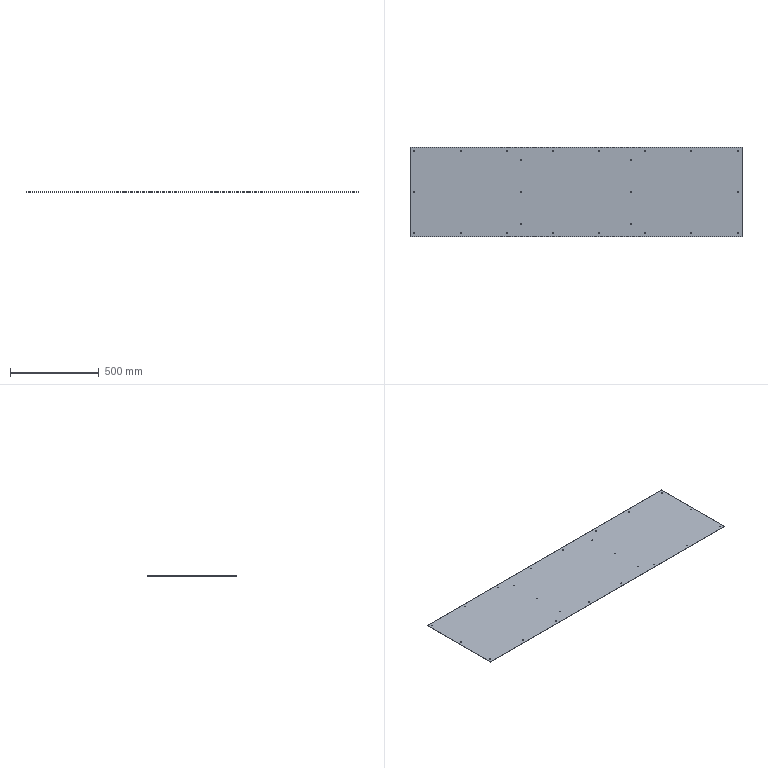Part | STEP file | TS-S93 | 1 solid | 54 faces | box 1870 x 502 x 1.2 mm | volume 1125828 mm3 | cylinder 48 | plane 6 | commonest cylinder face diameters 5.4 x48